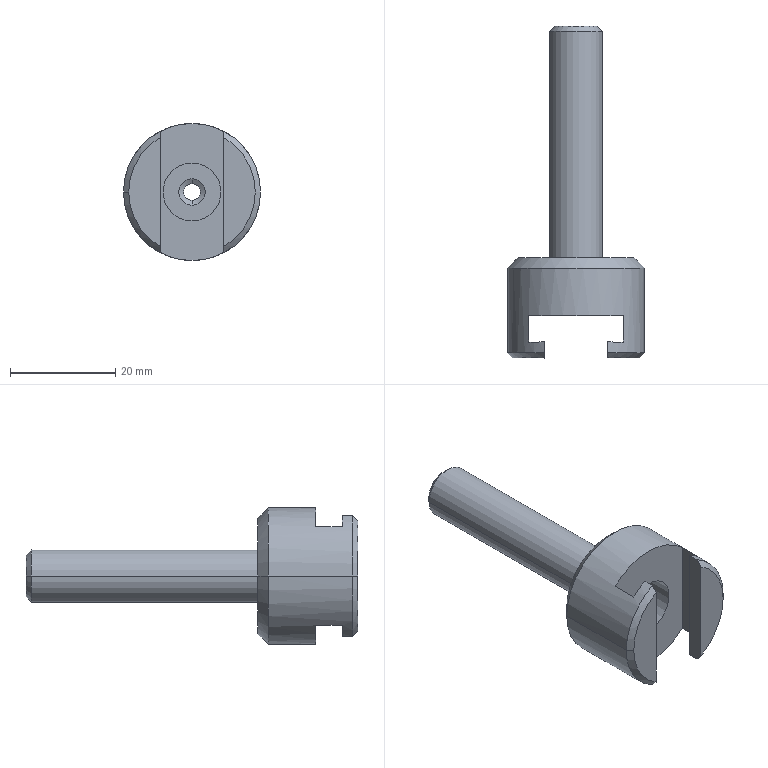Part | STEP file | BU-A07#180 | 1 solid | 31 faces | box 26 x 63 x 26 mm | volume 8732 mm3 | plane 12 | cylinder 10 | cone 9 | commonest cylinder face diameters 3.2 x2 5 x2 10 x2 11 x2 26 x2